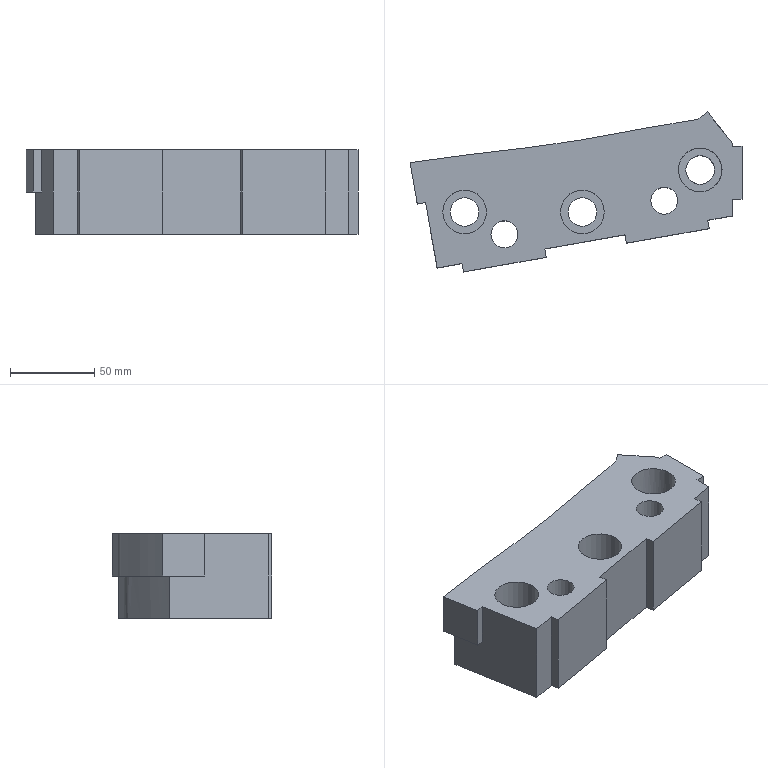Part | NX | features solid 2 | 1 solid | 34 faces | box 197.345 x 95.07 x 50 mm | volume 493508 mm3 | plane 24 | cylinder 8 | spline 2 | commonest cylinder face diameters 17 x3 26 x3 16 x2
STEP:
#1=CARTESIAN_POINT('',(141.996,549.553,0.));
#2=VERTEX_POINT('',#1);
#3=CARTESIAN_POINT('',(141.996,549.553,-25.));
#4=VERTEX_POINT('',#3);
#5=CARTESIAN_POINT('',(141.996,549.553,-50.));
#6=DIRECTION('',(0.,0.,-1.));
#7=VECTOR('',#6,1000.);
#8=LINE('',#5,#7);
#9=EDGE_CURVE('',#2,#4,#8,.T.);
#10=ORIENTED_EDGE('',*,*,#9,.F.);
#11=CARTESIAN_POINT('',(137.655,574.174,0.));
#12=VERTEX_POINT('',#11);
#13=CARTESIAN_POINT('',(148.858,510.637,0.));
#14=DIRECTION('',(-0.1736,0.9848,0.));
#15=VECTOR('',#14,1000.);
#16=LINE('',#13,#15);
#17=EDGE_CURVE('',#2,#12,#16,.T.);
#18=ORIENTED_EDGE('',*,*,#17,.T.);
#19=CARTESIAN_POINT('',(137.655,574.174,-25.));
#20=VERTEX_POINT('',#19);
#21=CARTESIAN_POINT('',(137.655,574.174,-50.));
#22=DIRECTION('',(0.,0.,1.));
#23=VECTOR('',#22,1000.);
#24=LINE('',#21,#23);
#25=EDGE_CURVE('',#20,#12,#24,.T.);
#26=ORIENTED_EDGE('',*,*,#25,.F.);
#27=CARTESIAN_POINT('',(148.858,510.637,-25.));
#28=DIRECTION('',(0.1736,-0.9848,0.));
#29=VECTOR('',#28,1000.);
#30=LINE('',#27,#29);
#31=EDGE_CURVE('',#20,#4,#30,.T.);
#32=ORIENTED_EDGE('',*,*,#31,.T.);
#33=EDGE_LOOP('',(#10,#18,#26,#32));
#34=FACE_BOUND('',#33,.T.);
#35=CARTESIAN_POINT('',(148.858,510.637,-50.));
#36=DIRECTION('',(0.9848,0.1736,0.));
#37=DIRECTION('',(-0.1736,0.9848,0.));
#38=AXIS2_PLACEMENT_3D('',#35,#36,#37);
#39=PLANE('',#38);
#40=ADVANCED_FACE('',(#34),#39,.F.);
#41=CARTESIAN_POINT('',(296.782,551.506,0.));
#42=VERTEX_POINT('',#41);
#43=CARTESIAN_POINT('',(288.782,551.506,0.));
#44=DIRECTION('',(0.,0.,1.));
#45=DIRECTION('',(1.,0.,0.));
#46=AXIS2_PLACEMENT_3D('',#43,#44,#45);
#47=CIRCLE('',#46,8.);
#48=EDGE_CURVE('',#42,#42,#47,.T.);
#49=ORIENTED_EDGE('',*,*,#48,.F.);
#50=EDGE_LOOP('',(#49));
#51=FACE_BOUND('',#50,.T.);
#52=CARTESIAN_POINT('',(201.782,531.506,0.));
#53=VERTEX_POINT('',#52);
#54=CARTESIAN_POINT('',(193.782,531.506,0.));
#55=DIRECTION('',(0.,0.,1.));
#56=DIRECTION('',(1.,0.,0.));
#57=AXIS2_PLACEMENT_3D('',#54,#55,#56);
#58=CIRCLE('',#57,8.);
#59=EDGE_CURVE('',#53,#53,#58,.T.);
#60=ORIENTED_EDGE('',*,*,#59,.F.);
#61=EDGE_LOOP('',(#60));
#62=FACE_BOUND('',#61,.T.);
#63=CARTESIAN_POINT('',(183.122,544.794,0.));
#64=VERTEX_POINT('',#63);
#65=CARTESIAN_POINT('',(170.122,544.794,0.));
#66=DIRECTION('',(0.,0.,1.));
#67=DIRECTION('',(1.,0.,0.));
#68=AXIS2_PLACEMENT_3D('',#65,#66,#67);
#69=CIRCLE('',#68,13.);
#70=EDGE_CURVE('',#64,#64,#69,.T.);
#71=ORIENTED_EDGE('',*,*,#70,.F.);
#72=EDGE_LOOP('',(#71));
#73=FACE_BOUND('',#72,.T.);
#74=CARTESIAN_POINT('',(253.122,544.794,0.));
#75=VERTEX_POINT('',#74);
#76=CARTESIAN_POINT('',(240.122,544.794,0.));
#77=DIRECTION('',(0.,0.,1.));
#78=DIRECTION('',(1.,0.,0.));
#79=AXIS2_PLACEMENT_3D('',#76,#77,#78);
#80=CIRCLE('',#79,13.);
#81=EDGE_CURVE('',#75,#75,#80,.T.);
#82=ORIENTED_EDGE('',*,*,#81,.F.);
#83=EDGE_LOOP('',(#82));
#84=FACE_BOUND('',#83,.T.);
#85=CARTESIAN_POINT('',(323.122,569.794,0.));
#86=VERTEX_POINT('',#85);
#87=CARTESIAN_POINT('',(310.122,569.794,0.));
#88=DIRECTION('',(0.,0.,1.));
#89=DIRECTION('',(1.,0.,0.));
#90=AXIS2_PLACEMENT_3D('',#87,#88,#89);
#91=CIRCLE('',#90,13.);
#92=EDGE_CURVE('',#86,#86,#91,.T.);
#93=ORIENTED_EDGE('',*,*,#92,.F.);
#94=EDGE_LOOP('',(#93));
#95=FACE_BOUND('',#94,.T.);
#96=ORIENTED_EDGE('',*,*,#17,.F.);
#97=CARTESIAN_POINT('',(146.92,550.422,0.));
#98=VERTEX_POINT('',#97);
#99=CARTESIAN_POINT('',(146.92,550.422,0.));
#100=DIRECTION('',(-0.9848,-0.1736,0.));
#101=VECTOR('',#100,1000.);
#102=LINE('',#99,#101);
#103=EDGE_CURVE('',#98,#2,#102,.T.);
#104=ORIENTED_EDGE('',*,*,#103,.F.);
#105=CARTESIAN_POINT('',(153.782,511.506,0.));
#106=VERTEX_POINT('',#105);
#107=CARTESIAN_POINT('',(153.782,511.506,0.));
#108=DIRECTION('',(-0.1736,0.9848,0.));
#109=VECTOR('',#108,1000.);
#110=LINE('',#107,#109);
#111=EDGE_CURVE('',#106,#98,#110,.T.);
#112=ORIENTED_EDGE('',*,*,#111,.F.);
#113=CARTESIAN_POINT('',(168.554,514.11,0.));
#114=VERTEX_POINT('',#113);
#115=CARTESIAN_POINT('',(329.431,542.477,0.));
#116=DIRECTION('',(-0.9848,-0.1736,0.));
#117=VECTOR('',#116,1000.);
#118=LINE('',#115,#117);
#119=EDGE_CURVE('',#114,#106,#118,.T.);
#120=ORIENTED_EDGE('',*,*,#119,.F.);
#121=CARTESIAN_POINT('',(169.422,509.186,0.));
#122=VERTEX_POINT('',#121);
#123=CARTESIAN_POINT('',(168.554,514.11,0.));
#124=DIRECTION('',(0.1736,-0.9848,0.));
#125=VECTOR('',#124,1000.);
#126=LINE('',#123,#125);
#127=EDGE_CURVE('',#114,#122,#126,.T.);
#128=ORIENTED_EDGE('',*,*,#127,.T.);
#129=CARTESIAN_POINT('',(218.663,517.869,0.));
#130=VERTEX_POINT('',#129);
#131=CARTESIAN_POINT('',(218.663,517.869,0.));
#132=DIRECTION('',(-0.9848,-0.1736,0.));
#133=VECTOR('',#132,1000.);
#134=LINE('',#131,#133);
#135=EDGE_CURVE('',#130,#122,#134,.T.);
#136=ORIENTED_EDGE('',*,*,#135,.F.);
#137=CARTESIAN_POINT('',(217.795,522.793,0.));
#138=VERTEX_POINT('',#137);
#139=CARTESIAN_POINT('',(217.795,522.793,0.));
#140=DIRECTION('',(0.1736,-0.9848,0.));
#141=VECTOR('',#140,1000.);
#142=LINE('',#139,#141);
#143=EDGE_CURVE('',#138,#130,#142,.T.);
#144=ORIENTED_EDGE('',*,*,#143,.F.);
#145=CARTESIAN_POINT('',(265.418,531.19,0.));
#146=VERTEX_POINT('',#145);
#147=CARTESIAN_POINT('',(329.431,542.477,0.));
#148=DIRECTION('',(-0.9848,-0.1736,0.));
#149=VECTOR('',#148,1000.);
#150=LINE('',#147,#149);
#151=EDGE_CURVE('',#146,#138,#150,.T.);
#152=ORIENTED_EDGE('',*,*,#151,.F.);
#153=CARTESIAN_POINT('',(266.286,526.266,0.));
#154=VERTEX_POINT('',#153);
#155=CARTESIAN_POINT('',(265.418,531.19,0.));
#156=DIRECTION('',(0.1736,-0.9848,0.));
#157=VECTOR('',#156,1000.);
#158=LINE('',#155,#157);
#159=EDGE_CURVE('',#146,#154,#158,.T.);
#160=ORIENTED_EDGE('',*,*,#159,.T.);
#161=CARTESIAN_POINT('',(315.527,534.949,0.));
#162=VERTEX_POINT('',#161);
#163=CARTESIAN_POINT('',(330.299,537.553,0.));
#164=DIRECTION('',(-0.9848,-0.1736,0.));
#165=VECTOR('',#164,1000.);
#166=LINE('',#163,#165);
#167=EDGE_CURVE('',#162,#154,#166,.T.);
#168=ORIENTED_EDGE('',*,*,#167,.F.);
#169=CARTESIAN_POINT('',(314.659,539.873,0.));
#170=VERTEX_POINT('',#169);
#171=CARTESIAN_POINT('',(314.659,539.873,0.));
#172=DIRECTION('',(0.1736,-0.9848,0.));
#173=VECTOR('',#172,1000.);
#174=LINE('',#171,#173);
#175=EDGE_CURVE('',#170,#162,#174,.T.);
#176=ORIENTED_EDGE('',*,*,#175,.F.);
#177=CARTESIAN_POINT('',(329.431,542.477,0.));
#178=VERTEX_POINT('',#177);
#179=CARTESIAN_POINT('',(329.431,542.477,0.));
#180=DIRECTION('',(-0.9848,-0.1736,0.));
#181=VECTOR('',#180,1000.);
#182=LINE('',#179,#181);
#183=EDGE_CURVE('',#178,#170,#182,.T.);
#184=ORIENTED_EDGE('',*,*,#183,.F.);
#185=CARTESIAN_POINT('',(329.431,552.501,0.));
#186=VERTEX_POINT('',#185);
#187=CARTESIAN_POINT('',(329.431,585.716,0.));
#188=DIRECTION('',(0.,-1.,0.));
#189=VECTOR('',#188,1000.);
#190=LINE('',#187,#189);
#191=EDGE_CURVE('',#186,#178,#190,.T.);
#192=ORIENTED_EDGE('',*,*,#191,.F.);
#193=CARTESIAN_POINT('',(335.,552.501,0.));
#194=VERTEX_POINT('',#193);
#195=CARTESIAN_POINT('',(334.431,552.501,0.));
#196=DIRECTION('',(1.,0.,0.));
#197=VECTOR('',#196,1000.);
#198=LINE('',#195,#197);
#199=EDGE_CURVE('',#194,#186,#198,.F.);
#200=ORIENTED_EDGE('',*,*,#199,.F.);
#201=CARTESIAN_POINT('',(335.,583.896,0.));
#202=VERTEX_POINT('',#201);
#203=CARTESIAN_POINT('',(335.,588.896,0.));
#204=DIRECTION('',(0.,-1.,0.));
#205=VECTOR('',#204,1000.);
#206=LINE('',#203,#205);
#207=EDGE_CURVE('',#202,#194,#206,.T.);
#208=ORIENTED_EDGE('',*,*,#207,.F.);
#209=CARTESIAN_POINT('',(329.431,583.896,0.));
#210=VERTEX_POINT('',#209);
#211=CARTESIAN_POINT('',(334.431,583.896,0.));
#212=DIRECTION('',(1.,0.,0.));
#213=VECTOR('',#212,1000.);
#214=LINE('',#211,#213);
#215=EDGE_CURVE('',#202,#210,#214,.F.);
#216=ORIENTED_EDGE('',*,*,#215,.T.);
#217=CARTESIAN_POINT('',(329.431,585.716,0.));
#218=VERTEX_POINT('',#217);
#219=CARTESIAN_POINT('',(329.431,585.716,0.));
#220=DIRECTION('',(0.,-1.,0.));
#221=VECTOR('',#220,1000.);
#222=LINE('',#219,#221);
#223=EDGE_CURVE('',#218,#210,#222,.T.);
#224=ORIENTED_EDGE('',*,*,#223,.F.);
#225=CARTESIAN_POINT('',(314.417,604.257,0.));
#226=VERTEX_POINT('',#225);
#227=CARTESIAN_POINT('',(329.431,585.716,0.));
#228=DIRECTION('',(-0.6293,0.7771,0.));
#229=VECTOR('',#228,1000.);
#230=LINE('',#227,#229);
#231=EDGE_CURVE('',#218,#226,#230,.T.);
#232=ORIENTED_EDGE('',*,*,#231,.T.);
#233=CARTESIAN_POINT('',(314.417,604.257,0.));
#234=CARTESIAN_POINT('',(313.456,603.513,0.));
#235=CARTESIAN_POINT('',(311.997,602.42,0.));
#236=CARTESIAN_POINT('',(310.125,600.866,0.));
#237=CARTESIAN_POINT('',(308.006,599.638,0.));
#238=CARTESIAN_POINT('',(304.985,599.087,0.));
#239=CARTESIAN_POINT('',(297.755,598.23,0.));
#240=CARTESIAN_POINT('',(282.167,595.571,0.));
#241=CARTESIAN_POINT('',(258.333,590.865,0.));
#242=CARTESIAN_POINT('',(229.601,585.825,0.));
#243=CARTESIAN_POINT('',(200.669,582.121,0.));
#244=CARTESIAN_POINT('',(171.683,578.904,0.));
#245=CARTESIAN_POINT('',(150.69,576.131,0.));
#246=CARTESIAN_POINT('',(139.366,574.434,0.));
#247=CARTESIAN_POINT('',(137.655,574.174,0.));
#248=B_SPLINE_CURVE_WITH_KNOTS('',3,(#233,#234,#235,#236,#237,#238,#239,#240,#241,#242,#243,#244,#245,#246,#247),.UNSPECIFIED.,.F.,.F.,(4,1,1,1,1,1,1,1,1,1,1,1,4),(0.,0.02023,0.03035,0.04047,0.0607,0.08093,0.1619,0.3237,0.4856,0.6475,0.8093,0.9712,1.),.UNSPECIFIED.);
#249=EDGE_CURVE('',#226,#12,#248,.T.);
#250=ORIENTED_EDGE('',*,*,#249,.T.);
#251=EDGE_LOOP('',(#96,#104,#112,#120,#128,#136,#144,#152,#160,#168,#176,#184,#192,#200,#208,#216,#224,#232,#250));
#252=FACE_BOUND('',#251,.T.);
#253=CARTESIAN_POINT('',(227.,585.664,0.));
#254=DIRECTION('',(0.,0.,1.));
#255=DIRECTION('',(1.,0.,0.));
#256=AXIS2_PLACEMENT_3D('',#253,#254,#255);
#257=PLANE('',#256);
#258=ADVANCED_FACE('',(#51,#62,#73,#84,#95,#252),#257,.T.);
#259=CARTESIAN_POINT('',(146.92,550.422,-25.));
#260=VERTEX_POINT('',#259);
#261=CARTESIAN_POINT('',(146.92,550.422,-25.));
#262=DIRECTION('',(-0.9848,-0.1736,0.));
#263=VECTOR('',#262,1000.);
#264=LINE('',#261,#263);
#265=EDGE_CURVE('',#260,#4,#264,.T.);
#266=ORIENTED_EDGE('',*,*,#265,.T.);
#267=ORIENTED_EDGE('',*,*,#31,.F.);
#268=CARTESIAN_POINT('',(314.417,604.257,-25.));
#269=VERTEX_POINT('',#268);
#270=CARTESIAN_POINT('',(314.417,604.257,-25.));
#271=CARTESIAN_POINT('',(313.456,603.513,-25.));
#272=CARTESIAN_POINT('',(311.997,602.42,-25.));
#273=CARTESIAN_POINT('',(310.125,600.866,-25.));
#274=CARTESIAN_POINT('',(308.006,599.638,-25.));
#275=CARTESIAN_POINT('',(304.985,599.087,-25.));
#276=CARTESIAN_POINT('',(297.755,598.23,-25.));
#277=CARTESIAN_POINT('',(282.167,595.571,-25.));
#278=CARTESIAN_POINT('',(258.333,590.865,-25.));
#279=CARTESIAN_POINT('',(229.601,585.825,-25.));
#280=CARTESIAN_POINT('',(200.669,582.121,-25.));
#281=CARTESIAN_POINT('',(171.683,578.904,-25.));
#282=CARTESIAN_POINT('',(150.69,576.131,-25.));
#283=CARTESIAN_POINT('',(139.366,574.434,-25.));
#284=CARTESIAN_POINT('',(137.655,574.174,-25.));
#285=B_SPLINE_CURVE_WITH_KNOTS('',3,(#270,#271,#272,#273,#274,#275,#276,#277,#278,#279,#280,#281,#282,#283,#284),.UNSPECIFIED.,.F.,.F.,(4,1,1,1,1,1,1,1,1,1,1,1,4),(0.,0.02023,0.03035,0.04047,0.0607,0.08093,0.1619,0.3237,0.4856,0.6475,0.8093,0.9712,1.),.UNSPECIFIED.);
#286=EDGE_CURVE('',#20,#269,#285,.F.);
#287=ORIENTED_EDGE('',*,*,#286,.T.);
#288=CARTESIAN_POINT('',(317.564,600.37,-25.));
#289=VERTEX_POINT('',#288);
#290=CARTESIAN_POINT('',(329.431,585.716,-25.));
#291=DIRECTION('',(0.6293,-0.7771,0.));
#292=VECTOR('',#291,1000.);
#293=LINE('',#290,#292);
#294=EDGE_CURVE('',#269,#289,#293,.T.);
#295=ORIENTED_EDGE('',*,*,#294,.T.);
#296=CARTESIAN_POINT('',(143.47,569.989,-25.));
#297=VERTEX_POINT('',#296);
#298=CARTESIAN_POINT('',(317.564,600.37,-25.));
#299=CARTESIAN_POINT('',(316.843,599.812,-25.));
#300=CARTESIAN_POINT('',(315.683,598.934,-25.));
#301=CARTESIAN_POINT('',(314.472,597.971,-25.));
#302=CARTESIAN_POINT('',(313.16,596.906,-25.));
#303=CARTESIAN_POINT('',(311.364,595.765,-25.));
#304=CARTESIAN_POINT('',(309.287,594.91,-25.));
#305=CARTESIAN_POINT('',(307.42,594.453,-25.));
#306=CARTESIAN_POINT('',(305.282,594.1,-25.));
#307=CARTESIAN_POINT('',(302.976,593.812,-25.));
#308=CARTESIAN_POINT('',(300.35,593.473,-25.));
#309=CARTESIAN_POINT('',(297.704,593.087,-25.));
#310=CARTESIAN_POINT('',(294.17,592.532,-25.));
#311=CARTESIAN_POINT('',(289.729,591.769,-25.));
#312=CARTESIAN_POINT('',(284.367,590.798,-25.));
#313=CARTESIAN_POINT('',(279.008,589.801,-25.));
#314=CARTESIAN_POINT('',(271.853,588.445,-25.));
#315=CARTESIAN_POINT('',(262.89,586.728,-25.));
#316=CARTESIAN_POINT('',(252.083,584.721,-25.));
#317=CARTESIAN_POINT('',(241.242,582.826,-25.));
#318=CARTESIAN_POINT('',(226.722,580.494,-25.));
#319=CARTESIAN_POINT('',(208.521,578.055,-25.));
#320=CARTESIAN_POINT('',(186.722,575.548,-25.));
#321=CARTESIAN_POINT('',(165.049,573.008,-25.));
#322=CARTESIAN_POINT('',(150.653,571.046,-25.));
#323=CARTESIAN_POINT('',(143.47,569.989,-25.));
#324=B_SPLINE_CURVE_WITH_KNOTS('',3,(#298,#299,#300,#301,#302,#303,#304,#305,#306,#307,#308,#309,#310,#311,#312,#313,#314,#315,#316,#317,#318,#319,#320,#321,#322,#323),.UNSPECIFIED.,.F.,.F.,(4,1,1,1,1,1,1,1,1,1,1,1,1,1,1,1,1,1,1,1,1,1,1,4),(-0.000619,0.01457,0.02216,0.02976,0.03735,0.04495,0.05254,0.06014,0.07532,0.09051,0.1057,0.1209,0.1513,0.1816,0.212,0.2424,0.3032,0.3639,0.4247,0.4854,0.6069,0.7284,0.8499,0.9714),.UNSPECIFIED.);
#325=EDGE_CURVE('',#289,#297,#324,.T.);
#326=ORIENTED_EDGE('',*,*,#325,.T.);
#327=CARTESIAN_POINT('',(153.782,511.506,-25.));
#328=DIRECTION('',(0.1736,-0.9848,0.));
#329=VECTOR('',#328,1000.);
#330=LINE('',#327,#329);
#331=EDGE_CURVE('',#260,#297,#330,.F.);
#332=ORIENTED_EDGE('',*,*,#331,.F.);
#333=EDGE_LOOP('',(#266,#267,#287,#295,#326,#332));
#334=FACE_BOUND('',#333,.T.);
#335=CARTESIAN_POINT('',(314.417,604.257,-25.));
#336=DIRECTION('',(0.,0.,1.));
#337=DIRECTION('',(1.,0.,0.));
#338=AXIS2_PLACEMENT_3D('',#335,#336,#337);
#339=PLANE('',#338);
#340=ADVANCED_FACE('',(#334),#339,.F.);
#341=CARTESIAN_POINT('',(329.431,583.896,-50.));
#342=VERTEX_POINT('',#341);
#343=CARTESIAN_POINT('',(329.431,583.896,-50.));
#344=DIRECTION('',(0.,0.,-1.));
#345=VECTOR('',#344,1000.);
#346=LINE('',#343,#345);
#347=EDGE_CURVE('',#342,#210,#346,.F.);
#348=ORIENTED_EDGE('',*,*,#347,.F.);
#349=CARTESIAN_POINT('',(329.431,585.716,-50.));
#350=VERTEX_POINT('',#349);
#351=CARTESIAN_POINT('',(329.431,585.716,-50.));
#352=DIRECTION('',(0.,-1.,0.));
#353=VECTOR('',#352,1000.);
#354=LINE('',#351,#353);
#355=EDGE_CURVE('',#350,#342,#354,.T.);
#356=ORIENTED_EDGE('',*,*,#355,.F.);
#357=CARTESIAN_POINT('',(329.431,585.716,-50.));
#358=DIRECTION('',(0.,0.,1.));
#359=VECTOR('',#358,1000.);
#360=LINE('',#357,#359);
#361=EDGE_CURVE('',#350,#218,#360,.T.);
#362=ORIENTED_EDGE('',*,*,#361,.T.);
#363=ORIENTED_EDGE('',*,*,#223,.T.);
#364=EDGE_LOOP('',(#348,#356,#362,#363));
#365=FACE_BOUND('',#364,.T.);
#366=CARTESIAN_POINT('',(329.431,585.716,-50.));
#367=DIRECTION('',(-1.,0.,0.));
#368=DIRECTION('',(0.,-1.,0.));
#369=AXIS2_PLACEMENT_3D('',#366,#367,#368);
#370=PLANE('',#369);
#371=ADVANCED_FACE('',(#365),#370,.F.);
#372=CARTESIAN_POINT('',(265.418,531.19,-50.));
#373=VERTEX_POINT('',#372);
#374=CARTESIAN_POINT('',(265.418,531.19,-50.));
#375=DIRECTION('',(0.,0.,1.));
#376=VECTOR('',#375,1000.);
#377=LINE('',#374,#376);
#378=EDGE_CURVE('',#373,#146,#377,.T.);
#379=ORIENTED_EDGE('',*,*,#378,.T.);
#380=ORIENTED_EDGE('',*,*,#151,.T.);
#381=CARTESIAN_POINT('',(217.795,522.793,-50.));
#382=VERTEX_POINT('',#381);
#383=CARTESIAN_POINT('',(217.795,522.793,-50.));
#384=DIRECTION('',(0.,0.,1.));
#385=VECTOR('',#384,1000.);
#386=LINE('',#383,#385);
#387=EDGE_CURVE('',#382,#138,#386,.T.);
#388=ORIENTED_EDGE('',*,*,#387,.F.);
#389=CARTESIAN_POINT('',(329.431,542.477,-50.));
#390=DIRECTION('',(-0.9848,-0.1736,0.));
#391=VECTOR('',#390,1000.);
#392=LINE('',#389,#391);
#393=EDGE_CURVE('',#373,#382,#392,.T.);
#394=ORIENTED_EDGE('',*,*,#393,.F.);
#395=EDGE_LOOP('',(#379,#380,#388,#394));
#396=FACE_BOUND('',#395,.T.);
#397=CARTESIAN_POINT('',(329.431,542.477,-50.));
#398=DIRECTION('',(-0.1736,0.9848,0.));
#399=DIRECTION('',(-0.9848,-0.1736,0.));
#400=AXIS2_PLACEMENT_3D('',#397,#398,#399);
#401=PLANE('',#400);
#402=ADVANCED_FACE('',(#396),#401,.F.);
#403=ORIENTED_EDGE('',*,*,#119,.T.);
#404=CARTESIAN_POINT('',(153.782,511.506,-50.));
#405=VERTEX_POINT('',#404);
#406=CARTESIAN_POINT('',(153.782,511.506,-50.));
#407=DIRECTION('',(0.,0.,1.));
#408=VECTOR('',#407,1000.);
#409=LINE('',#406,#408);
#410=EDGE_CURVE('',#405,#106,#409,.T.);
#411=ORIENTED_EDGE('',*,*,#410,.F.);
#412=CARTESIAN_POINT('',(168.554,514.11,-50.));
#413=VERTEX_POINT('',#412);
#414=CARTESIAN_POINT('',(329.431,542.477,-50.));
#415=DIRECTION('',(-0.9848,-0.1736,0.));
#416=VECTOR('',#415,1000.);
#417=LINE('',#414,#416);
#418=EDGE_CURVE('',#413,#405,#417,.T.);
#419=ORIENTED_EDGE('',*,*,#418,.F.);
#420=CARTESIAN_POINT('',(168.554,514.11,-50.));
#421=DIRECTION('',(0.,0.,1.));
#422=VECTOR('',#421,1000.);
#423=LINE('',#420,#422);
#424=EDGE_CURVE('',#413,#114,#423,.T.);
#425=ORIENTED_EDGE('',*,*,#424,.T.);
#426=EDGE_LOOP('',(#403,#411,#419,#425));
#427=FACE_BOUND('',#426,.T.);
#428=CARTESIAN_POINT('',(329.431,542.477,-50.));
#429=DIRECTION('',(-0.1736,0.9848,0.));
#430=DIRECTION('',(-0.9848,-0.1736,0.));
#431=AXIS2_PLACEMENT_3D('',#428,#429,#430);
#432=PLANE('',#431);
#433=ADVANCED_FACE('',(#427),#432,.F.);
#434=CARTESIAN_POINT('',(296.782,551.506,-50.));
#435=VERTEX_POINT('',#434);
#436=CARTESIAN_POINT('',(288.782,551.506,-50.));
#437=DIRECTION('',(0.,0.,1.));
#438=DIRECTION('',(1.,0.,0.));
#439=AXIS2_PLACEMENT_3D('',#436,#437,#438);
#440=CIRCLE('',#439,8.);
#441=EDGE_CURVE('',#435,#435,#440,.T.);
#442=ORIENTED_EDGE('',*,*,#441,.T.);
#443=EDGE_LOOP('',(#442));
#444=FACE_BOUND('',#443,.T.);
#445=CARTESIAN_POINT('',(201.782,531.506,-50.));
#446=VERTEX_POINT('',#445);
#447=CARTESIAN_POINT('',(193.782,531.506,-50.));
#448=DIRECTION('',(0.,0.,1.));
#449=DIRECTION('',(1.,0.,0.));
#450=AXIS2_PLACEMENT_3D('',#447,#448,#449);
#451=CIRCLE('',#450,8.);
#452=EDGE_CURVE('',#446,#446,#451,.T.);
#453=ORIENTED_EDGE('',*,*,#452,.T.);
#454=EDGE_LOOP('',(#453));
#455=FACE_BOUND('',#454,.T.);
#456=CARTESIAN_POINT('',(318.622,569.794,-50.));
#457=VERTEX_POINT('',#456);
#458=CARTESIAN_POINT('',(310.122,569.794,-50.));
#459=DIRECTION('',(0.,0.,1.));
#460=DIRECTION('',(1.,0.,0.));
#461=AXIS2_PLACEMENT_3D('',#458,#459,#460);
#462=CIRCLE('',#461,8.5);
#463=EDGE_CURVE('',#457,#457,#462,.T.);
#464=ORIENTED_EDGE('',*,*,#463,.T.);
#465=EDGE_LOOP('',(#464));
#466=FACE_BOUND('',#465,.T.);
#467=CARTESIAN_POINT('',(248.622,544.794,-50.));
#468=VERTEX_POINT('',#467);
#469=CARTESIAN_POINT('',(240.122,544.794,-50.));
#470=DIRECTION('',(0.,0.,1.));
#471=DIRECTION('',(1.,0.,0.));
#472=AXIS2_PLACEMENT_3D('',#469,#470,#471);
#473=CIRCLE('',#472,8.5);
#474=EDGE_CURVE('',#468,#468,#473,.T.);
#475=ORIENTED_EDGE('',*,*,#474,.T.);
#476=EDGE_LOOP('',(#475));
#477=FACE_BOUND('',#476,.T.);
#478=CARTESIAN_POINT('',(178.622,544.794,-50.));
#479=VERTEX_POINT('',#478);
#480=CARTESIAN_POINT('',(170.122,544.794,-50.));
#481=DIRECTION('',(0.,0.,1.));
#482=DIRECTION('',(1.,0.,0.));
#483=AXIS2_PLACEMENT_3D('',#480,#481,#482);
#484=CIRCLE('',#483,8.5);
#485=EDGE_CURVE('',#479,#479,#484,.T.);
#486=ORIENTED_EDGE('',*,*,#485,.T.);
#487=EDGE_LOOP('',(#486));
#488=FACE_BOUND('',#487,.T.);
#489=CARTESIAN_POINT('',(143.47,569.989,-50.));
#490=VERTEX_POINT('',#489);
#491=CARTESIAN_POINT('',(143.308,570.907,-50.));
#492=DIRECTION('',(0.1736,-0.9848,0.));
#493=VECTOR('',#492,1000.);
#494=LINE('',#491,#493);
#495=EDGE_CURVE('',#490,#405,#494,.T.);
#496=ORIENTED_EDGE('',*,*,#495,.F.);
#497=CARTESIAN_POINT('',(317.564,600.37,-50.));
#498=VERTEX_POINT('',#497);
#499=CARTESIAN_POINT('',(143.47,569.989,-50.));
#500=CARTESIAN_POINT('',(145.224,570.247,-50.));
#501=CARTESIAN_POINT('',(148.774,570.76,-50.));
#502=CARTESIAN_POINT('',(153.311,571.391,-50.));
#503=CARTESIAN_POINT('',(157.,571.89,-50.));
#504=CARTESIAN_POINT('',(159.8,572.262,-50.));
#505=CARTESIAN_POINT('',(162.148,572.568,-50.));
#506=CARTESIAN_POINT('',(163.826,572.783,-50.));
#507=CARTESIAN_POINT('',(164.754,572.902,-50.));
#508=CARTESIAN_POINT('',(165.55,573.003,-50.));
#509=CARTESIAN_POINT('',(165.974,573.057,-50.));
#510=CARTESIAN_POINT('',(166.688,573.146,-50.));
#511=CARTESIAN_POINT('',(167.917,573.3,-50.));
#512=CARTESIAN_POINT('',(169.826,573.536,-50.));
#513=CARTESIAN_POINT('',(172.294,573.837,-50.));
#514=CARTESIAN_POINT('',(175.843,574.264,-50.));
#515=CARTESIAN_POINT('',(180.773,574.848,-50.));
#516=CARTESIAN_POINT('',(186.279,575.489,-50.));
#517=CARTESIAN_POINT('',(191.204,576.059,-50.));
#518=CARTESIAN_POINT('',(195.638,576.577,-50.));
#519=CARTESIAN_POINT('',(199.647,577.05,-50.));
#520=CARTESIAN_POINT('',(203.164,577.47,-50.));
#521=CARTESIAN_POINT('',(205.167,577.712,-50.));
#522=CARTESIAN_POINT('',(206.65,577.893,-50.));
#523=CARTESIAN_POINT('',(207.701,578.022,-50.));
#524=CARTESIAN_POINT('',(208.535,578.126,-50.));
#525=CARTESIAN_POINT('',(209.077,578.193,-50.));
#526=CARTESIAN_POINT('',(209.404,578.234,-50.));
#527=CARTESIAN_POINT('',(209.577,578.256,-50.));
#528=CARTESIAN_POINT('',(210.01,578.311,-50.));
#529=CARTESIAN_POINT('',(210.495,578.372,-50.));
#530=CARTESIAN_POINT('',(211.383,578.484,-50.));
#531=CARTESIAN_POINT('',(212.617,578.642,-50.));
#532=CARTESIAN_POINT('',(214.091,578.833,-50.));
#533=CARTESIAN_POINT('',(216.029,579.086,-50.));
#534=CARTESIAN_POINT('',(218.409,579.403,-50.));
#535=CARTESIAN_POINT('',(222.121,579.91,-50.));
#536=CARTESIAN_POINT('',(226.607,580.547,-50.));
#537=CARTESIAN_POINT('',(231.611,581.295,-50.));
#538=CARTESIAN_POINT('',(236.701,582.098,-50.));
#539=CARTESIAN_POINT('',(241.173,582.837,-50.));
#540=CARTESIAN_POINT('',(244.861,583.466,-50.));
#541=CARTESIAN_POINT('',(247.688,583.958,-50.));
#542=CARTESIAN_POINT('',(250.086,584.382,-50.));
#543=CARTESIAN_POINT('',(251.805,584.691,-50.));
#544=CARTESIAN_POINT('',(252.772,584.865,-50.));
#545=CARTESIAN_POINT('',(253.565,585.009,-50.));
#546=CARTESIAN_POINT('',(254.116,585.109,-50.));
#547=CARTESIAN_POINT('',(254.952,585.261,-50.));
#548=CARTESIAN_POINT('',(256.412,585.529,-50.));
#549=CARTESIAN_POINT('',(258.62,585.938,-50.));
#550=CARTESIAN_POINT('',(260.974,586.378,-50.));
#551=CARTESIAN_POINT('',(262.912,586.742,-50.));
#552=CARTESIAN_POINT('',(264.49,587.041,-50.));
#553=CARTESIAN_POINT('',(265.797,587.289,-50.));
#554=CARTESIAN_POINT('',(267.635,587.637,-50.));
#555=CARTESIAN_POINT('',(269.897,588.067,-50.));
#556=CARTESIAN_POINT('',(272.182,588.502,-50.));
#557=CARTESIAN_POINT('',(273.757,588.803,-50.));
#558=CARTESIAN_POINT('',(274.692,588.981,-50.));
#559=CARTESIAN_POINT('',(275.294,589.096,-50.));
#560=CARTESIAN_POINT('',(276.277,589.284,-50.));
#561=CARTESIAN_POINT('',(277.431,589.503,-50.));
#562=CARTESIAN_POINT('',(279.467,589.888,-50.));
#563=CARTESIAN_POINT('',(282.201,590.4,-50.));
#564=CARTESIAN_POINT('',(285.273,590.965,-50.));
#565=CARTESIAN_POINT('',(288.117,591.478,-50.));
#566=CARTESIAN_POINT('',(290.74,591.94,-50.));
#567=CARTESIAN_POINT('',(293.135,592.35,-50.));
#568=CARTESIAN_POINT('',(294.957,592.651,-50.));
#569=CARTESIAN_POINT('',(296.111,592.836,-50.));
#570=CARTESIAN_POINT('',(296.78,592.94,-50.));
#571=CARTESIAN_POINT('',(297.163,593.,-50.));
#572=CARTESIAN_POINT('',(297.931,593.116,-50.));
#573=CARTESIAN_POINT('',(298.82,593.248,-50.));
#574=CARTESIAN_POINT('',(299.983,593.415,-50.));
#575=CARTESIAN_POINT('',(301.114,593.569,-50.));
#576=CARTESIAN_POINT('',(302.057,593.693,-50.));
#577=CARTESIAN_POINT('',(302.669,593.771,-50.));
#578=CARTESIAN_POINT('',(303.648,593.896,-50.));
#579=CARTESIAN_POINT('',(304.375,593.991,-50.));
#580=CARTESIAN_POINT('',(304.892,594.061,-50.));
#581=CARTESIAN_POINT('',(305.27,594.114,-50.));
#582=CARTESIAN_POINT('',(305.433,594.137,-50.));
#583=CARTESIAN_POINT('',(305.907,594.208,-50.));
#584=CARTESIAN_POINT('',(306.4,594.288,-50.));
#585=CARTESIAN_POINT('',(307.005,594.393,-50.));
#586=CARTESIAN_POINT('',(307.663,594.526,-50.));
#587=CARTESIAN_POINT('',(308.177,594.643,-50.));
#588=CARTESIAN_POINT('',(308.894,594.838,-50.));
#589=CARTESIAN_POINT('',(309.755,595.121,-50.));
#590=CARTESIAN_POINT('',(310.827,595.559,-50.));
#591=CARTESIAN_POINT('',(312.018,596.178,-50.));
#592=CARTESIAN_POINT('',(313.051,596.861,-50.));
#593=CARTESIAN_POINT('',(313.656,597.318,-50.));
#594=CARTESIAN_POINT('',(314.273,597.807,-50.));
#595=CARTESIAN_POINT('',(314.941,598.344,-50.));
#596=CARTESIAN_POINT('',(315.334,598.654,-50.));
#597=CARTESIAN_POINT('',(315.922,599.111,-50.));
#598=CARTESIAN_POINT('',(316.64,599.665,-50.));
#599=CARTESIAN_POINT('',(317.196,600.09,-50.));
#600=CARTESIAN_POINT('',(317.564,600.37,-50.));
#601=B_SPLINE_CURVE_WITH_KNOTS('',3,(#499,#500,#501,#502,#503,#504,#505,#506,#507,#508,#509,#510,#511,#512,#513,#514,#515,#516,#517,#518,#519,#520,#521,#522,#523,#524,#525,#526,#527,#528,#529,#530,#531,#532,#533,#534,#535,#536,#537,#538,#539,#540,#541,#542,#543,#544,#545,#546,#547,#548,#549,#550,#551,#552,#553,#554,#555,#556,#557,#558,#559,#560,#561,#562,#563,#564,#565,#566,#567,#568,#569,#570,#571,#572,#573,#574,#575,#576,#577,#578,#579,#580,#581,#582,#583,#584,#585,#586,#587,#588,#589,#590,#591,#592,#593,#594,#595,#596,#597,#598,#599,#600),.UNSPECIFIED.,.F.,.F.,(4,1,1,1,1,1,1,1,1,1,1,1,1,1,1,1,1,1,1,1,1,1,1,1,1,1,1,1,1,1,1,1,1,1,1,1,1,1,1,1,1,1,1,1,1,1,1,1,1,1,1,1,1,1,1,1,1,1,1,1,1,1,1,1,1,1,1,1,1,1,1,1,1,1,1,1,1,1,1,1,1,1,1,1,1,1,1,1,1,1,1,1,1,1,1,1,1,1,1,4),(0.,0.03125,0.0625,0.07812,0.09375,0.1094,0.1172,0.1211,0.125,0.1289,0.1328,0.1406,0.1562,0.1719,0.1875,0.2188,0.25,0.2656,0.2812,0.3125,0.3281,0.3438,0.3516,0.3594,0.3672,0.3711,0.373,0.375,0.377,0.3789,0.3828,0.3906,0.3984,0.4062,0.4219,0.4375,0.4688,0.5,0.5312,0.5625,0.5781,0.5938,0.6094,0.6172,0.6211,0.625,0.6289,0.6328,0.6406,0.6562,0.6719,0.6797,0.6875,0.6953,0.7031,0.7188,0.7344,0.7422,0.7461,0.75,0.7539,0.7578,0.7656,0.7812,0.7969,0.8125,0.8281,0.8438,0.8594,0.8672,0.8711,0.875,0.8789,0.8828,0.8906,0.8984,0.9023,0.9062,0.9102,0.9141,0.918,0.9199,0.9219,0.9238,0.9258,0.9297,0.9336,0.9375,0.9414,0.9453,0.9531,0.9609,0.9688,0.9727,0.9766,0.9805,0.9844,0.9883,0.9922,1.),.UNSPECIFIED.);
#602=EDGE_CURVE('',#490,#498,#601,.T.);
#603=ORIENTED_EDGE('',*,*,#602,.T.);
#604=CARTESIAN_POINT('',(329.431,585.716,-50.));
#605=DIRECTION('',(-0.6293,0.7771,0.));
#606=VECTOR('',#605,1000.);
#607=LINE('',#604,#606);
#608=EDGE_CURVE('',#350,#498,#607,.T.);
#609=ORIENTED_EDGE('',*,*,#608,.F.);
#610=ORIENTED_EDGE('',*,*,#355,.T.);
#611=CARTESIAN_POINT('',(335.,583.896,-50.));
#612=VERTEX_POINT('',#611);
#613=CARTESIAN_POINT('',(334.431,583.896,-50.));
#614=DIRECTION('',(1.,0.,0.));
#615=VECTOR('',#614,1000.);
#616=LINE('',#613,#615);
#617=EDGE_CURVE('',#612,#342,#616,.F.);
#618=ORIENTED_EDGE('',*,*,#617,.F.);
#619=CARTESIAN_POINT('',(335.,552.501,-50.));
#620=VERTEX_POINT('',#619);
#621=CARTESIAN_POINT('',(335.,588.896,-50.));
#622=DIRECTION('',(0.,-1.,0.));
#623=VECTOR('',#622,1000.);
#624=LINE('',#621,#623);
#625=EDGE_CURVE('',#612,#620,#624,.T.);
#626=ORIENTED_EDGE('',*,*,#625,.T.);
#627=CARTESIAN_POINT('',(329.431,552.501,-50.));
#628=VERTEX_POINT('',#627);
#629=CARTESIAN_POINT('',(334.431,552.501,-50.));
#630=DIRECTION('',(1.,0.,0.));
#631=VECTOR('',#630,1000.);
#632=LINE('',#629,#631);
#633=EDGE_CURVE('',#620,#628,#632,.F.);
#634=ORIENTED_EDGE('',*,*,#633,.T.);
#635=CARTESIAN_POINT('',(329.431,542.477,-50.));
#636=VERTEX_POINT('',#635);
#637=CARTESIAN_POINT('',(329.431,585.716,-50.));
#638=DIRECTION('',(0.,-1.,0.));
#639=VECTOR('',#638,1000.);
#640=LINE('',#637,#639);
#641=EDGE_CURVE('',#628,#636,#640,.T.);
#642=ORIENTED_EDGE('',*,*,#641,.T.);
#643=CARTESIAN_POINT('',(314.659,539.873,-50.));
#644=VERTEX_POINT('',#643);
#645=CARTESIAN_POINT('',(329.431,542.477,-50.));
#646=DIRECTION('',(-0.9848,-0.1736,0.));
#647=VECTOR('',#646,1000.);
#648=LINE('',#645,#647);
#649=EDGE_CURVE('',#636,#644,#648,.T.);
#650=ORIENTED_EDGE('',*,*,#649,.T.);
#651=CARTESIAN_POINT('',(315.527,534.949,-50.));
#652=VERTEX_POINT('',#651);
#653=CARTESIAN_POINT('',(314.659,539.873,-50.));
#654=DIRECTION('',(0.1736,-0.9848,0.));
#655=VECTOR('',#654,1000.);
#656=LINE('',#653,#655);
#657=EDGE_CURVE('',#644,#652,#656,.T.);
#658=ORIENTED_EDGE('',*,*,#657,.T.);
#659=CARTESIAN_POINT('',(266.286,526.266,-50.));
#660=VERTEX_POINT('',#659);
#661=CARTESIAN_POINT('',(330.299,537.553,-50.));
#662=DIRECTION('',(-0.9848,-0.1736,0.));
#663=VECTOR('',#662,1000.);
#664=LINE('',#661,#663);
#665=EDGE_CURVE('',#652,#660,#664,.T.);
#666=ORIENTED_EDGE('',*,*,#665,.T.);
#667=CARTESIAN_POINT('',(265.418,531.19,-50.));
#668=DIRECTION('',(0.1736,-0.9848,0.));
#669=VECTOR('',#668,1000.);
#670=LINE('',#667,#669);
#671=EDGE_CURVE('',#373,#660,#670,.T.);
#672=ORIENTED_EDGE('',*,*,#671,.F.);
#673=ORIENTED_EDGE('',*,*,#393,.T.);
#674=CARTESIAN_POINT('',(218.663,517.869,-50.));
#675=VERTEX_POINT('',#674);
#676=CARTESIAN_POINT('',(217.795,522.793,-50.));
#677=DIRECTION('',(0.1736,-0.9848,0.));
#678=VECTOR('',#677,1000.);
#679=LINE('',#676,#678);
#680=EDGE_CURVE('',#382,#675,#679,.T.);
#681=ORIENTED_EDGE('',*,*,#680,.T.);
#682=CARTESIAN_POINT('',(169.422,509.186,-50.));
#683=VERTEX_POINT('',#682);
#684=CARTESIAN_POINT('',(218.663,517.869,-50.));
#685=DIRECTION('',(-0.9848,-0.1736,0.));
#686=VECTOR('',#685,1000.);
#687=LINE('',#684,#686);
#688=EDGE_CURVE('',#675,#683,#687,.T.);
#689=ORIENTED_EDGE('',*,*,#688,.T.);
#690=CARTESIAN_POINT('',(168.554,514.11,-50.));
#691=DIRECTION('',(0.1736,-0.9848,0.));
#692=VECTOR('',#691,1000.);
#693=LINE('',#690,#692);
#694=EDGE_CURVE('',#413,#683,#693,.T.);
#695=ORIENTED_EDGE('',*,*,#694,.F.);
#696=ORIENTED_EDGE('',*,*,#418,.T.);
#697=EDGE_LOOP('',(#496,#603,#609,#610,#618,#626,#634,#642,#650,#658,#666,#672,#673,#681,#689,#695,#696));
#698=FACE_BOUND('',#697,.T.);
#699=CARTESIAN_POINT('',(227.,585.664,-50.));
#700=DIRECTION('',(0.,0.,1.));
#701=DIRECTION('',(1.,0.,0.));
#702=AXIS2_PLACEMENT_3D('',#699,#700,#701);
#703=PLANE('',#702);
#704=ADVANCED_FACE('',(#444,#455,#466,#477,#488,#698),#703,.F.);
#705=CARTESIAN_POINT('',(143.47,569.989,-37.5));
#706=DIRECTION('',(0.,0.,-1.));
#707=VECTOR('',#706,1000.);
#708=LINE('',#705,#707);
#709=EDGE_CURVE('',#297,#490,#708,.T.);
#710=ORIENTED_EDGE('',*,*,#709,.F.);
#711=ORIENTED_EDGE('',*,*,#325,.F.);
#712=CARTESIAN_POINT('',(317.564,600.37,-42.5));
#713=DIRECTION('',(0.,0.,-1.));
#714=VECTOR('',#713,1000.);
#715=LINE('',#712,#714);
#716=EDGE_CURVE('',#289,#498,#715,.T.);
#717=ORIENTED_EDGE('',*,*,#716,.T.);
#718=ORIENTED_EDGE('',*,*,#602,.F.);
#719=EDGE_LOOP('',(#710,#711,#717,#718));
#720=FACE_BOUND('',#719,.T.);
#721=CARTESIAN_POINT('',(317.564,600.37,-25.));
#722=CARTESIAN_POINT('',(317.564,600.37,-50.));
#723=CARTESIAN_POINT('',(316.843,599.812,-25.));
#724=CARTESIAN_POINT('',(316.843,599.812,-50.));
#725=CARTESIAN_POINT('',(315.683,598.934,-25.));
#726=CARTESIAN_POINT('',(315.683,598.934,-50.));
#727=CARTESIAN_POINT('',(314.472,597.971,-25.));
#728=CARTESIAN_POINT('',(314.472,597.971,-50.));
#729=CARTESIAN_POINT('',(313.16,596.906,-25.));
#730=CARTESIAN_POINT('',(313.16,596.906,-50.));
#731=CARTESIAN_POINT('',(311.364,595.765,-25.));
#732=CARTESIAN_POINT('',(311.364,595.765,-50.));
#733=CARTESIAN_POINT('',(309.287,594.91,-25.));
#734=CARTESIAN_POINT('',(309.287,594.91,-50.));
#735=CARTESIAN_POINT('',(307.42,594.453,-25.));
#736=CARTESIAN_POINT('',(307.42,594.453,-50.));
#737=CARTESIAN_POINT('',(305.282,594.1,-25.));
#738=CARTESIAN_POINT('',(305.282,594.1,-50.));
#739=CARTESIAN_POINT('',(302.976,593.812,-25.));
#740=CARTESIAN_POINT('',(302.976,593.812,-50.));
#741=CARTESIAN_POINT('',(300.35,593.473,-25.));
#742=CARTESIAN_POINT('',(300.35,593.473,-50.));
#743=CARTESIAN_POINT('',(297.704,593.087,-25.));
#744=CARTESIAN_POINT('',(297.704,593.087,-50.));
#745=CARTESIAN_POINT('',(294.17,592.532,-25.));
#746=CARTESIAN_POINT('',(294.17,592.532,-50.));
#747=CARTESIAN_POINT('',(289.729,591.769,-25.));
#748=CARTESIAN_POINT('',(289.729,591.769,-50.));
#749=CARTESIAN_POINT('',(284.367,590.798,-25.));
#750=CARTESIAN_POINT('',(284.367,590.798,-50.));
#751=CARTESIAN_POINT('',(279.008,589.801,-25.));
#752=CARTESIAN_POINT('',(279.008,589.801,-50.));
#753=CARTESIAN_POINT('',(271.853,588.445,-25.));
#754=CARTESIAN_POINT('',(271.853,588.445,-50.));
#755=CARTESIAN_POINT('',(262.89,586.728,-25.));
#756=CARTESIAN_POINT('',(262.89,586.728,-50.));
#757=CARTESIAN_POINT('',(252.083,584.721,-25.));
#758=CARTESIAN_POINT('',(252.083,584.721,-50.));
#759=CARTESIAN_POINT('',(241.242,582.826,-25.));
#760=CARTESIAN_POINT('',(241.242,582.826,-50.));
#761=CARTESIAN_POINT('',(226.722,580.494,-25.));
#762=CARTESIAN_POINT('',(226.722,580.494,-50.));
#763=CARTESIAN_POINT('',(208.521,578.055,-25.));
#764=CARTESIAN_POINT('',(208.521,578.055,-50.));
#765=CARTESIAN_POINT('',(186.722,575.548,-25.));
#766=CARTESIAN_POINT('',(186.722,575.548,-50.));
#767=CARTESIAN_POINT('',(165.049,573.008,-25.));
#768=CARTESIAN_POINT('',(165.049,573.008,-50.));
#769=CARTESIAN_POINT('',(150.653,571.046,-25.));
#770=CARTESIAN_POINT('',(150.653,571.046,-50.));
#771=CARTESIAN_POINT('',(143.47,569.989,-25.));
#772=CARTESIAN_POINT('',(143.47,569.989,-50.));
#773=B_SPLINE_SURFACE_WITH_KNOTS('',3,1,((#721,#722),(#723,#724),(#725,#726),(#727,#728),(#729,#730),(#731,#732),(#733,#734),(#735,#736),(#737,#738),(#739,#740),(#741,#742),(#743,#744),(#745,#746),(#747,#748),(#749,#750),(#751,#752),(#753,#754),(#755,#756),(#757,#758),(#759,#760),(#761,#762),(#763,#764),(#765,#766),(#767,#768),(#769,#770),(#771,#772)),.SURF_OF_LINEAR_EXTRUSION.,.F.,.F.,.F.,(4,1,1,1,1,1,1,1,1,1,1,1,1,1,1,1,1,1,1,1,1,1,1,4),(2,2),(-0.000619,0.01457,0.02216,0.02976,0.03735,0.04495,0.05254,0.06014,0.07532,0.09051,0.1057,0.1209,0.1513,0.1816,0.212,0.2424,0.3032,0.3639,0.4247,0.4854,0.6069,0.7284,0.8499,0.9714),(0.,1.),.UNSPECIFIED.);
#774=ADVANCED_FACE('',(#720),#773,.F.);
#775=ORIENTED_EDGE('',*,*,#286,.F.);
#776=ORIENTED_EDGE('',*,*,#25,.T.);
#777=ORIENTED_EDGE('',*,*,#249,.F.);
#778=CARTESIAN_POINT('',(314.417,604.257,-50.));
#779=DIRECTION('',(0.,0.,1.));
#780=VECTOR('',#779,1000.);
#781=LINE('',#778,#780);
#782=EDGE_CURVE('',#269,#226,#781,.T.);
#783=ORIENTED_EDGE('',*,*,#782,.F.);
#784=EDGE_LOOP('',(#775,#776,#777,#783));
#785=FACE_BOUND('',#784,.T.);
#786=CARTESIAN_POINT('',(314.417,604.257,-25.));
#787=CARTESIAN_POINT('',(314.417,604.257,0.));
#788=CARTESIAN_POINT('',(313.675,603.682,-25.));
#789=CARTESIAN_POINT('',(313.675,603.682,0.));
#790=CARTESIAN_POINT('',(312.165,602.573,-25.));
#791=CARTESIAN_POINT('',(312.165,602.573,0.));
#792=CARTESIAN_POINT('',(310.031,600.706,-25.));
#793=CARTESIAN_POINT('',(310.031,600.706,0.));
#794=CARTESIAN_POINT('',(307.473,599.493,-25.));
#795=CARTESIAN_POINT('',(307.473,599.493,0.));
#796=CARTESIAN_POINT('',(304.66,599.066,-25.));
#797=CARTESIAN_POINT('',(304.66,599.066,0.));
#798=CARTESIAN_POINT('',(301.872,598.713,-25.));
#799=CARTESIAN_POINT('',(301.872,598.713,0.));
#800=CARTESIAN_POINT('',(298.154,598.222,-25.));
#801=CARTESIAN_POINT('',(298.154,598.222,0.));
#802=CARTESIAN_POINT('',(291.665,597.207,-25.));
#803=CARTESIAN_POINT('',(291.665,597.207,0.));
#804=CARTESIAN_POINT('',(282.423,595.535,-25.));
#805=CARTESIAN_POINT('',(282.423,595.535,0.));
#806=CARTESIAN_POINT('',(271.36,593.442,-25.));
#807=CARTESIAN_POINT('',(271.36,593.442,0.));
#808=CARTESIAN_POINT('',(260.302,591.325,-25.));
#809=CARTESIAN_POINT('',(260.302,591.325,0.));
#810=CARTESIAN_POINT('',(245.536,588.607,-25.));
#811=CARTESIAN_POINT('',(245.536,588.607,0.));
#812=CARTESIAN_POINT('',(227.019,585.534,-25.));
#813=CARTESIAN_POINT('',(227.019,585.534,0.));
#814=CARTESIAN_POINT('',(204.684,582.624,-25.));
#815=CARTESIAN_POINT('',(204.684,582.624,0.));
#816=CARTESIAN_POINT('',(174.845,579.25,-25.));
#817=CARTESIAN_POINT('',(174.845,579.25,0.));
#818=CARTESIAN_POINT('',(152.497,576.433,-25.));
#819=CARTESIAN_POINT('',(152.497,576.433,0.));
#820=CARTESIAN_POINT('',(137.655,574.174,-25.));
#821=CARTESIAN_POINT('',(137.655,574.174,0.));
#822=B_SPLINE_SURFACE_WITH_KNOTS('',3,1,((#786,#787),(#788,#789),(#790,#791),(#792,#793),(#794,#795),(#796,#797),(#798,#799),(#800,#801),(#802,#803),(#804,#805),(#806,#807),(#808,#809),(#810,#811),(#812,#813),(#814,#815),(#816,#817),(#818,#819),(#820,#821)),.SURF_OF_LINEAR_EXTRUSION.,.F.,.F.,.F.,(4,1,1,1,1,1,1,1,1,1,1,1,1,1,1,4),(2,2),(0.,0.01562,0.03125,0.04688,0.0625,0.07812,0.09375,0.125,0.1875,0.25,0.3125,0.375,0.5,0.625,0.75,1.),(0.,1.),.UNSPECIFIED.);
#823=ADVANCED_FACE('',(#785),#822,.T.);
#824=ORIENTED_EDGE('',*,*,#183,.T.);
#825=CARTESIAN_POINT('',(314.659,539.873,-50.));
#826=DIRECTION('',(0.,0.,1.));
#827=VECTOR('',#826,1000.);
#828=LINE('',#825,#827);
#829=EDGE_CURVE('',#644,#170,#828,.T.);
#830=ORIENTED_EDGE('',*,*,#829,.F.);
#831=ORIENTED_EDGE('',*,*,#649,.F.);
#832=CARTESIAN_POINT('',(329.431,542.477,-50.));
#833=DIRECTION('',(0.,0.,1.));
#834=VECTOR('',#833,1000.);
#835=LINE('',#832,#834);
#836=EDGE_CURVE('',#636,#178,#835,.T.);
#837=ORIENTED_EDGE('',*,*,#836,.T.);
#838=EDGE_LOOP('',(#824,#830,#831,#837));
#839=FACE_BOUND('',#838,.T.);
#840=CARTESIAN_POINT('',(329.431,542.477,-50.));
#841=DIRECTION('',(-0.1736,0.9848,0.));
#842=DIRECTION('',(-0.9848,-0.1736,0.));
#843=AXIS2_PLACEMENT_3D('',#840,#841,#842);
#844=PLANE('',#843);
#845=ADVANCED_FACE('',(#839),#844,.F.);
#846=ORIENTED_EDGE('',*,*,#641,.F.);
#847=CARTESIAN_POINT('',(329.431,552.501,-50.));
#848=DIRECTION('',(0.,0.,-1.));
#849=VECTOR('',#848,1000.);
#850=LINE('',#847,#849);
#851=EDGE_CURVE('',#628,#186,#850,.F.);
#852=ORIENTED_EDGE('',*,*,#851,.T.);
#853=ORIENTED_EDGE('',*,*,#191,.T.);
#854=ORIENTED_EDGE('',*,*,#836,.F.);
#855=EDGE_LOOP('',(#846,#852,#853,#854));
#856=FACE_BOUND('',#855,.T.);
#857=CARTESIAN_POINT('',(329.431,585.716,-50.));
#858=DIRECTION('',(-1.,0.,0.));
#859=DIRECTION('',(0.,-1.,0.));
#860=AXIS2_PLACEMENT_3D('',#857,#858,#859);
#861=PLANE('',#860);
#862=ADVANCED_FACE('',(#856),#861,.F.);
#863=ORIENTED_EDGE('',*,*,#294,.F.);
#864=ORIENTED_EDGE('',*,*,#782,.T.);
#865=ORIENTED_EDGE('',*,*,#231,.F.);
#866=ORIENTED_EDGE('',*,*,#361,.F.);
#867=ORIENTED_EDGE('',*,*,#608,.T.);
#868=ORIENTED_EDGE('',*,*,#716,.F.);
#869=EDGE_LOOP('',(#863,#864,#865,#866,#867,#868));
#870=FACE_BOUND('',#869,.T.);
#871=CARTESIAN_POINT('',(329.431,585.716,-50.));
#872=DIRECTION('',(0.7771,0.6293,0.));
#873=DIRECTION('',(-0.6293,0.7771,0.));
#874=AXIS2_PLACEMENT_3D('',#871,#872,#873);
#875=PLANE('',#874);
#876=ADVANCED_FACE('',(#870),#875,.T.);
#877=ORIENTED_EDGE('',*,*,#410,.T.);
#878=ORIENTED_EDGE('',*,*,#111,.T.);
#879=CARTESIAN_POINT('',(146.92,550.422,-50.));
#880=DIRECTION('',(0.,0.,1.));
#881=VECTOR('',#880,1000.);
#882=LINE('',#879,#881);
#883=EDGE_CURVE('',#260,#98,#882,.T.);
#884=ORIENTED_EDGE('',*,*,#883,.F.);
#885=ORIENTED_EDGE('',*,*,#331,.T.);
#886=ORIENTED_EDGE('',*,*,#709,.T.);
#887=ORIENTED_EDGE('',*,*,#495,.T.);
#888=EDGE_LOOP('',(#877,#878,#884,#885,#886,#887));
#889=FACE_BOUND('',#888,.T.);
#890=CARTESIAN_POINT('',(153.782,511.506,-25.));
#891=DIRECTION('',(-0.9848,-0.1736,0.));
#892=DIRECTION('',(0.1736,-0.9848,0.));
#893=AXIS2_PLACEMENT_3D('',#890,#891,#892);
#894=PLANE('',#893);
#895=ADVANCED_FACE('',(#889),#894,.T.);
#896=CARTESIAN_POINT('',(161.622,544.794,-25.));
#897=VERTEX_POINT('',#896);
#898=CARTESIAN_POINT('',(170.122,544.794,-25.));
#899=DIRECTION('',(0.,0.,-1.));
#900=DIRECTION('',(-1.,0.,0.));
#901=AXIS2_PLACEMENT_3D('',#898,#899,#900);
#902=CIRCLE('',#901,8.5);
#903=EDGE_CURVE('',#897,#897,#902,.F.);
#904=ORIENTED_EDGE('',*,*,#903,.T.);
#905=EDGE_LOOP('',(#904));
#906=FACE_BOUND('',#905,.T.);
#907=ORIENTED_EDGE('',*,*,#485,.F.);
#908=EDGE_LOOP('',(#907));
#909=FACE_BOUND('',#908,.T.);
#910=CARTESIAN_POINT('',(170.122,544.794,-75.));
#911=DIRECTION('',(0.,0.,1.));
#912=DIRECTION('',(1.,0.,0.));
#913=AXIS2_PLACEMENT_3D('',#910,#911,#912);
#914=CYLINDRICAL_SURFACE('',#913,8.5);
#915=ADVANCED_FACE('',(#906,#909),#914,.F.);
#916=ORIENTED_EDGE('',*,*,#903,.F.);
#917=EDGE_LOOP('',(#916));
#918=FACE_BOUND('',#917,.T.);
#919=CARTESIAN_POINT('',(183.122,544.794,-25.));
#920=VERTEX_POINT('',#919);
#921=CARTESIAN_POINT('',(170.122,544.794,-25.));
#922=DIRECTION('',(0.,0.,1.));
#923=DIRECTION('',(1.,0.,0.));
#924=AXIS2_PLACEMENT_3D('',#921,#922,#923);
#925=CIRCLE('',#924,13.);
#926=EDGE_CURVE('',#920,#920,#925,.T.);
#927=ORIENTED_EDGE('',*,*,#926,.T.);
#928=EDGE_LOOP('',(#927));
#929=FACE_BOUND('',#928,.T.);
#930=CARTESIAN_POINT('',(170.122,544.794,-25.));
#931=DIRECTION('',(0.,0.,-1.));
#932=DIRECTION('',(-1.,0.,0.));
#933=AXIS2_PLACEMENT_3D('',#930,#931,#932);
#934=PLANE('',#933);
#935=ADVANCED_FACE('',(#918,#929),#934,.F.);
#936=ORIENTED_EDGE('',*,*,#70,.T.);
#937=EDGE_LOOP('',(#936));
#938=FACE_BOUND('',#937,.T.);
#939=ORIENTED_EDGE('',*,*,#926,.F.);
#940=EDGE_LOOP('',(#939));
#941=FACE_BOUND('',#940,.T.);
#942=CARTESIAN_POINT('',(170.122,544.794,-25.));
#943=DIRECTION('',(0.,0.,1.));
#944=DIRECTION('',(1.,0.,0.));
#945=AXIS2_PLACEMENT_3D('',#942,#943,#944);
#946=CYLINDRICAL_SURFACE('',#945,13.);
#947=ADVANCED_FACE('',(#938,#941),#946,.F.);
#948=CARTESIAN_POINT('',(231.622,544.794,-25.));
#949=VERTEX_POINT('',#948);
#950=CARTESIAN_POINT('',(240.122,544.794,-25.));
#951=DIRECTION('',(0.,0.,-1.));
#952=DIRECTION('',(-1.,0.,0.));
#953=AXIS2_PLACEMENT_3D('',#950,#951,#952);
#954=CIRCLE('',#953,8.5);
#955=EDGE_CURVE('',#949,#949,#954,.F.);
#956=ORIENTED_EDGE('',*,*,#955,.T.);
#957=EDGE_LOOP('',(#956));
#958=FACE_BOUND('',#957,.T.);
#959=ORIENTED_EDGE('',*,*,#474,.F.);
#960=EDGE_LOOP('',(#959));
#961=FACE_BOUND('',#960,.T.);
#962=CARTESIAN_POINT('',(240.122,544.794,-75.));
#963=DIRECTION('',(0.,0.,1.));
#964=DIRECTION('',(1.,0.,0.));
#965=AXIS2_PLACEMENT_3D('',#962,#963,#964);
#966=CYLINDRICAL_SURFACE('',#965,8.5);
#967=ADVANCED_FACE('',(#958,#961),#966,.F.);
#968=ORIENTED_EDGE('',*,*,#955,.F.);
#969=EDGE_LOOP('',(#968));
#970=FACE_BOUND('',#969,.T.);
#971=CARTESIAN_POINT('',(253.122,544.794,-25.));
#972=VERTEX_POINT('',#971);
#973=CARTESIAN_POINT('',(240.122,544.794,-25.));
#974=DIRECTION('',(0.,0.,1.));
#975=DIRECTION('',(1.,0.,0.));
#976=AXIS2_PLACEMENT_3D('',#973,#974,#975);
#977=CIRCLE('',#976,13.);
#978=EDGE_CURVE('',#972,#972,#977,.T.);
#979=ORIENTED_EDGE('',*,*,#978,.T.);
#980=EDGE_LOOP('',(#979));
#981=FACE_BOUND('',#980,.T.);
#982=CARTESIAN_POINT('',(240.122,544.794,-25.));
#983=DIRECTION('',(0.,0.,-1.));
#984=DIRECTION('',(-1.,0.,0.));
#985=AXIS2_PLACEMENT_3D('',#982,#983,#984);
#986=PLANE('',#985);
#987=ADVANCED_FACE('',(#970,#981),#986,.F.);
#988=ORIENTED_EDGE('',*,*,#81,.T.);
#989=EDGE_LOOP('',(#988));
#990=FACE_BOUND('',#989,.T.);
#991=ORIENTED_EDGE('',*,*,#978,.F.);
#992=EDGE_LOOP('',(#991));
#993=FACE_BOUND('',#992,.T.);
#994=CARTESIAN_POINT('',(240.122,544.794,-25.));
#995=DIRECTION('',(0.,0.,1.));
#996=DIRECTION('',(1.,0.,0.));
#997=AXIS2_PLACEMENT_3D('',#994,#995,#996);
#998=CYLINDRICAL_SURFACE('',#997,13.);
#999=ADVANCED_FACE('',(#990,#993),#998,.F.);
#1000=CARTESIAN_POINT('',(310.122,578.294,-25.));
#1001=VERTEX_POINT('',#1000);
#1002=CARTESIAN_POINT('',(310.122,569.794,-25.));
#1003=DIRECTION('',(0.,0.,-1.));
#1004=DIRECTION('',(0.,1.,0.));
#1005=AXIS2_PLACEMENT_3D('',#1002,#1003,#1004);
#1006=CIRCLE('',#1005,8.5);
#1007=EDGE_CURVE('',#1001,#1001,#1006,.F.);
#1008=ORIENTED_EDGE('',*,*,#1007,.T.);
#1009=EDGE_LOOP('',(#1008));
#1010=FACE_BOUND('',#1009,.T.);
#1011=ORIENTED_EDGE('',*,*,#463,.F.);
#1012=EDGE_LOOP('',(#1011));
#1013=FACE_BOUND('',#1012,.T.);
#1014=CARTESIAN_POINT('',(310.122,569.794,-75.));
#1015=DIRECTION('',(0.,0.,1.));
#1016=DIRECTION('',(0.,-1.,0.));
#1017=AXIS2_PLACEMENT_3D('',#1014,#1015,#1016);
#1018=CYLINDRICAL_SURFACE('',#1017,8.5);
#1019=ADVANCED_FACE('',(#1010,#1013),#1018,.F.);
#1020=ORIENTED_EDGE('',*,*,#1007,.F.);
#1021=EDGE_LOOP('',(#1020));
#1022=FACE_BOUND('',#1021,.T.);
#1023=CARTESIAN_POINT('',(310.122,556.794,-25.));
#1024=VERTEX_POINT('',#1023);
#1025=CARTESIAN_POINT('',(310.122,569.794,-25.));
#1026=DIRECTION('',(0.,0.,1.));
#1027=DIRECTION('',(0.,-1.,0.));
#1028=AXIS2_PLACEMENT_3D('',#1025,#1026,#1027);
#1029=CIRCLE('',#1028,13.);
#1030=EDGE_CURVE('',#1024,#1024,#1029,.T.);
#1031=ORIENTED_EDGE('',*,*,#1030,.T.);
#1032=EDGE_LOOP('',(#1031));
#1033=FACE_BOUND('',#1032,.T.);
#1034=CARTESIAN_POINT('',(310.122,569.794,-25.));
#1035=DIRECTION('',(0.,0.,-1.));
#1036=DIRECTION('',(0.,1.,0.));
#1037=AXIS2_PLACEMENT_3D('',#1034,#1035,#1036);
#1038=PLANE('',#1037);
#1039=ADVANCED_FACE('',(#1022,#1033),#1038,.F.);
#1040=ORIENTED_EDGE('',*,*,#92,.T.);
#1041=EDGE_LOOP('',(#1040));
#1042=FACE_BOUND('',#1041,.T.);
#1043=ORIENTED_EDGE('',*,*,#1030,.F.);
#1044=EDGE_LOOP('',(#1043));
#1045=FACE_BOUND('',#1044,.T.);
#1046=CARTESIAN_POINT('',(310.122,569.794,-25.));
#1047=DIRECTION('',(0.,0.,1.));
#1048=DIRECTION('',(0.,-1.,0.));
#1049=AXIS2_PLACEMENT_3D('',#1046,#1047,#1048);
#1050=CYLINDRICAL_SURFACE('',#1049,13.);
#1051=ADVANCED_FACE('',(#1042,#1045),#1050,.F.);
#1052=CARTESIAN_POINT('',(169.422,509.186,-50.));
#1053=DIRECTION('',(0.,0.,1.));
#1054=VECTOR('',#1053,1000.);
#1055=LINE('',#1052,#1054);
#1056=EDGE_CURVE('',#683,#122,#1055,.T.);
#1057=ORIENTED_EDGE('',*,*,#1056,.T.);
#1058=ORIENTED_EDGE('',*,*,#127,.F.);
#1059=ORIENTED_EDGE('',*,*,#424,.F.);
#1060=ORIENTED_EDGE('',*,*,#694,.T.);
#1061=EDGE_LOOP('',(#1057,#1058,#1059,#1060));
#1062=FACE_BOUND('',#1061,.T.);
#1063=CARTESIAN_POINT('',(168.554,514.11,-50.));
#1064=DIRECTION('',(0.9848,0.1736,0.));
#1065=DIRECTION('',(-0.1736,0.9848,0.));
#1066=AXIS2_PLACEMENT_3D('',#1063,#1064,#1065);
#1067=PLANE('',#1066);
#1068=ADVANCED_FACE('',(#1062),#1067,.F.);
#1069=CARTESIAN_POINT('',(218.663,517.869,-50.));
#1070=DIRECTION('',(0.,0.,1.));
#1071=VECTOR('',#1070,1000.);
#1072=LINE('',#1069,#1071);
#1073=EDGE_CURVE('',#675,#130,#1072,.T.);
#1074=ORIENTED_EDGE('',*,*,#1073,.F.);
#1075=ORIENTED_EDGE('',*,*,#680,.F.);
#1076=ORIENTED_EDGE('',*,*,#387,.T.);
#1077=ORIENTED_EDGE('',*,*,#143,.T.);
#1078=EDGE_LOOP('',(#1074,#1075,#1076,#1077));
#1079=FACE_BOUND('',#1078,.T.);
#1080=CARTESIAN_POINT('',(217.795,522.793,-50.));
#1081=DIRECTION('',(0.9848,0.1736,0.));
#1082=DIRECTION('',(-0.1736,0.9848,0.));
#1083=AXIS2_PLACEMENT_3D('',#1080,#1081,#1082);
#1084=PLANE('',#1083);
#1085=ADVANCED_FACE('',(#1079),#1084,.T.);
#1086=ORIENTED_EDGE('',*,*,#135,.T.);
#1087=ORIENTED_EDGE('',*,*,#1056,.F.);
#1088=ORIENTED_EDGE('',*,*,#688,.F.);
#1089=ORIENTED_EDGE('',*,*,#1073,.T.);
#1090=EDGE_LOOP('',(#1086,#1087,#1088,#1089));
#1091=FACE_BOUND('',#1090,.T.);
#1092=CARTESIAN_POINT('',(218.663,517.869,-50.));
#1093=DIRECTION('',(-0.1736,0.9848,0.));
#1094=DIRECTION('',(-0.9848,-0.1736,0.));
#1095=AXIS2_PLACEMENT_3D('',#1092,#1093,#1094);
#1096=PLANE('',#1095);
#1097=ADVANCED_FACE('',(#1091),#1096,.F.);
#1098=CARTESIAN_POINT('',(266.286,526.266,-50.));
#1099=DIRECTION('',(0.,0.,1.));
#1100=VECTOR('',#1099,1000.);
#1101=LINE('',#1098,#1100);
#1102=EDGE_CURVE('',#660,#154,#1101,.T.);
#1103=ORIENTED_EDGE('',*,*,#1102,.T.);
#1104=ORIENTED_EDGE('',*,*,#159,.F.);
#1105=ORIENTED_EDGE('',*,*,#378,.F.);
#1106=ORIENTED_EDGE('',*,*,#671,.T.);
#1107=EDGE_LOOP('',(#1103,#1104,#1105,#1106));
#1108=FACE_BOUND('',#1107,.T.);
#1109=CARTESIAN_POINT('',(265.418,531.19,-50.));
#1110=DIRECTION('',(0.9848,0.1736,0.));
#1111=DIRECTION('',(-0.1736,0.9848,0.));
#1112=AXIS2_PLACEMENT_3D('',#1109,#1110,#1111);
#1113=PLANE('',#1112);
#1114=ADVANCED_FACE('',(#1108),#1113,.F.);
#1115=CARTESIAN_POINT('',(315.527,534.949,-50.));
#1116=DIRECTION('',(0.,0.,1.));
#1117=VECTOR('',#1116,1000.);
#1118=LINE('',#1115,#1117);
#1119=EDGE_CURVE('',#652,#162,#1118,.T.);
#1120=ORIENTED_EDGE('',*,*,#1119,.F.);
#1121=ORIENTED_EDGE('',*,*,#657,.F.);
#1122=ORIENTED_EDGE('',*,*,#829,.T.);
#1123=ORIENTED_EDGE('',*,*,#175,.T.);
#1124=EDGE_LOOP('',(#1120,#1121,#1122,#1123));
#1125=FACE_BOUND('',#1124,.T.);
#1126=CARTESIAN_POINT('',(314.659,539.873,-50.));
#1127=DIRECTION('',(0.9848,0.1736,0.));
#1128=DIRECTION('',(-0.1736,0.9848,0.));
#1129=AXIS2_PLACEMENT_3D('',#1126,#1127,#1128);
#1130=PLANE('',#1129);
#1131=ADVANCED_FACE('',(#1125),#1130,.T.);
#1132=ORIENTED_EDGE('',*,*,#167,.T.);
#1133=ORIENTED_EDGE('',*,*,#1102,.F.);
#1134=ORIENTED_EDGE('',*,*,#665,.F.);
#1135=ORIENTED_EDGE('',*,*,#1119,.T.);
#1136=EDGE_LOOP('',(#1132,#1133,#1134,#1135));
#1137=FACE_BOUND('',#1136,.T.);
#1138=CARTESIAN_POINT('',(330.299,537.553,-50.));
#1139=DIRECTION('',(-0.1736,0.9848,0.));
#1140=DIRECTION('',(-0.9848,-0.1736,0.));
#1141=AXIS2_PLACEMENT_3D('',#1138,#1139,#1140);
#1142=PLANE('',#1141);
#1143=ADVANCED_FACE('',(#1137),#1142,.F.);
#1144=ORIENTED_EDGE('',*,*,#851,.F.);
#1145=ORIENTED_EDGE('',*,*,#633,.F.);
#1146=CARTESIAN_POINT('',(335.,552.501,-50.));
#1147=DIRECTION('',(0.,0.,-1.));
#1148=VECTOR('',#1147,1000.);
#1149=LINE('',#1146,#1148);
#1150=EDGE_CURVE('',#620,#194,#1149,.F.);
#1151=ORIENTED_EDGE('',*,*,#1150,.T.);
#1152=ORIENTED_EDGE('',*,*,#199,.T.);
#1153=EDGE_LOOP('',(#1144,#1145,#1151,#1152));
#1154=FACE_BOUND('',#1153,.T.);
#1155=CARTESIAN_POINT('',(334.431,552.501,-50.));
#1156=DIRECTION('',(0.,1.,0.));
#1157=DIRECTION('',(0.,0.,1.));
#1158=AXIS2_PLACEMENT_3D('',#1155,#1156,#1157);
#1159=PLANE('',#1158);
#1160=ADVANCED_FACE('',(#1154),#1159,.F.);
#1161=ORIENTED_EDGE('',*,*,#347,.T.);
#1162=ORIENTED_EDGE('',*,*,#215,.F.);
#1163=CARTESIAN_POINT('',(335.,583.896,-50.));
#1164=DIRECTION('',(0.,0.,-1.));
#1165=VECTOR('',#1164,1000.);
#1166=LINE('',#1163,#1165);
#1167=EDGE_CURVE('',#612,#202,#1166,.F.);
#1168=ORIENTED_EDGE('',*,*,#1167,.F.);
#1169=ORIENTED_EDGE('',*,*,#617,.T.);
#1170=EDGE_LOOP('',(#1161,#1162,#1168,#1169));
#1171=FACE_BOUND('',#1170,.T.);
#1172=CARTESIAN_POINT('',(334.431,583.896,-50.));
#1173=DIRECTION('',(0.,1.,0.));
#1174=DIRECTION('',(0.,0.,1.));
#1175=AXIS2_PLACEMENT_3D('',#1172,#1173,#1174);
#1176=PLANE('',#1175);
#1177=ADVANCED_FACE('',(#1171),#1176,.T.);
#1178=ORIENTED_EDGE('',*,*,#207,.T.);
#1179=ORIENTED_EDGE('',*,*,#1150,.F.);
#1180=ORIENTED_EDGE('',*,*,#625,.F.);
#1181=ORIENTED_EDGE('',*,*,#1167,.T.);
#1182=EDGE_LOOP('',(#1178,#1179,#1180,#1181));
#1183=FACE_BOUND('',#1182,.T.);
#1184=CARTESIAN_POINT('',(335.,588.896,-50.));
#1185=DIRECTION('',(-1.,0.,0.));
#1186=DIRECTION('',(0.,-1.,0.));
#1187=AXIS2_PLACEMENT_3D('',#1184,#1185,#1186);
#1188=PLANE('',#1187);
#1189=ADVANCED_FACE('',(#1183),#1188,.F.);
#1190=ORIENTED_EDGE('',*,*,#9,.T.);
#1191=ORIENTED_EDGE('',*,*,#265,.F.);
#1192=ORIENTED_EDGE('',*,*,#883,.T.);
#1193=ORIENTED_EDGE('',*,*,#103,.T.);
#1194=EDGE_LOOP('',(#1190,#1191,#1192,#1193));
#1195=FACE_BOUND('',#1194,.T.);
#1196=CARTESIAN_POINT('',(146.92,550.422,-50.));
#1197=DIRECTION('',(0.1736,-0.9848,0.));
#1198=DIRECTION('',(0.9848,0.1736,0.));
#1199=AXIS2_PLACEMENT_3D('',#1196,#1197,#1198);
#1200=PLANE('',#1199);
#1201=ADVANCED_FACE('',(#1195),#1200,.T.);
#1202=ORIENTED_EDGE('',*,*,#59,.T.);
#1203=EDGE_LOOP('',(#1202));
#1204=FACE_BOUND('',#1203,.T.);
#1205=ORIENTED_EDGE('',*,*,#452,.F.);
#1206=EDGE_LOOP('',(#1205));
#1207=FACE_BOUND('',#1206,.T.);
#1208=CARTESIAN_POINT('',(193.782,531.506,50.));
#1209=DIRECTION('',(0.,0.,-1.));
#1210=DIRECTION('',(-1.,0.,0.));
#1211=AXIS2_PLACEMENT_3D('',#1208,#1209,#1210);
#1212=CYLINDRICAL_SURFACE('',#1211,8.);
#1213=ADVANCED_FACE('',(#1204,#1207),#1212,.F.);
#1214=ORIENTED_EDGE('',*,*,#48,.T.);
#1215=EDGE_LOOP('',(#1214));
#1216=FACE_BOUND('',#1215,.T.);
#1217=ORIENTED_EDGE('',*,*,#441,.F.);
#1218=EDGE_LOOP('',(#1217));
#1219=FACE_BOUND('',#1218,.T.);
#1220=CARTESIAN_POINT('',(288.782,551.506,50.));
#1221=DIRECTION('',(0.,0.,-1.));
#1222=DIRECTION('',(-1.,0.,0.));
#1223=AXIS2_PLACEMENT_3D('',#1220,#1221,#1222);
#1224=CYLINDRICAL_SURFACE('',#1223,8.);
#1225=ADVANCED_FACE('',(#1216,#1219),#1224,.F.);
#1226=CLOSED_SHELL('',(#40,#258,#340,#371,#402,#433,#704,#774,#823,#845,#862,#876,#895,#915,#935,#947,#967,#987,#999,#1019,#1039,#1051,#1068,#1085,#1097,#1114,#1131,#1143,#1160,#1177,#1189,#1201,#1213,#1225));
#1227=MANIFOLD_SOLID_BREP('',#1226);
#1228=(LENGTH_UNIT()NAMED_UNIT(*)SI_UNIT(.MILLI.,.METRE.));
#1229=UNCERTAINTY_MEASURE_WITH_UNIT(LENGTH_MEASURE(0.0508),#1228,'','');
#1230=(NAMED_UNIT(*)PLANE_ANGLE_UNIT()SI_UNIT($,.RADIAN.));
#1231=(NAMED_UNIT(*)SI_UNIT($,.STERADIAN.)SOLID_ANGLE_UNIT());
#1232=(GEOMETRIC_REPRESENTATION_CONTEXT(3)GLOBAL_UNCERTAINTY_ASSIGNED_CONTEXT((#1229))GLOBAL_UNIT_ASSIGNED_CONTEXT((#1228,#1230,#1231))REPRESENTATION_CONTEXT('',''));
#1233=ADVANCED_BREP_SHAPE_REPRESENTATION('',(#1227),#1232);